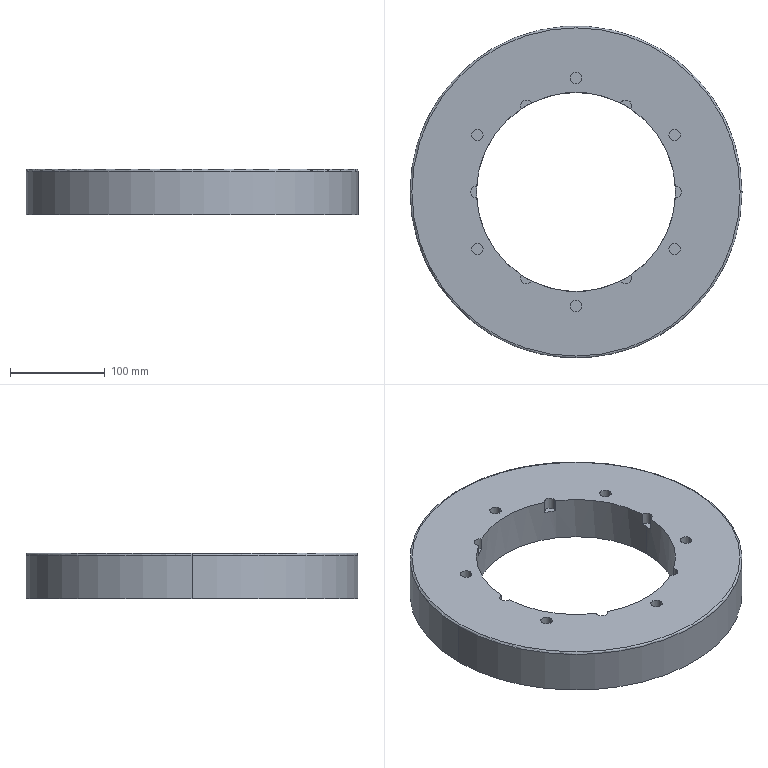Part | SolidWorks | features HoleWzd 3, Revolution 1 | 1 solid | 59 faces | box 350 x 350 x 48 mm | volume 2905895 mm3 | cylinder 37 | plane 20 | torus 2 | commonest cylinder face diameters 12 x21 16.4 x12 210 x2 350 x2